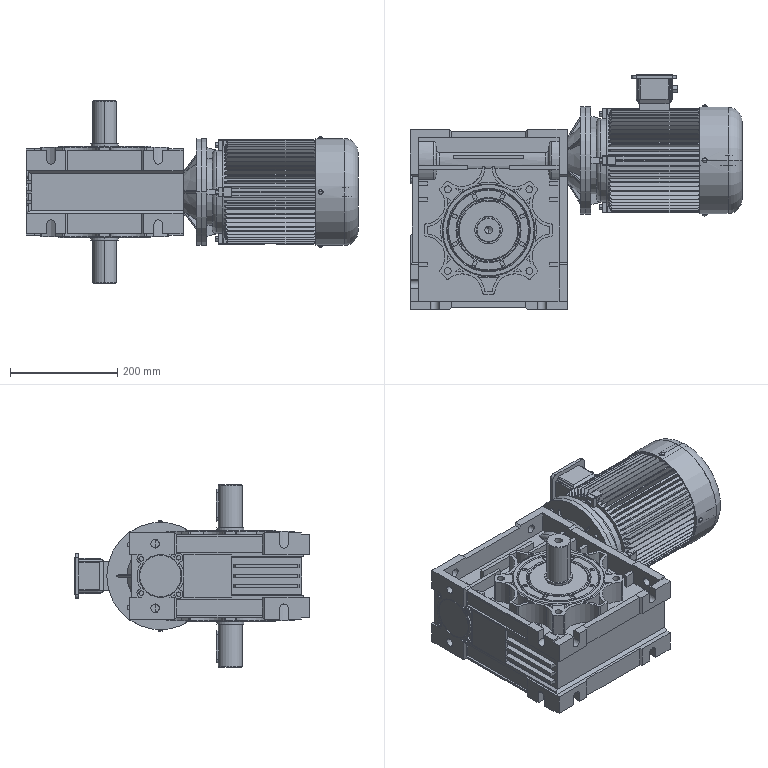Part | SolidWorks | 4 solids | 1490 faces | box 618.25 x 437.5 x 340 mm | volume 18932676 mm3 | plane 882 | cylinder 368 | cone 190 | torus 42 | sphere 8 | commonest cylinder face diameters 5.184 x42 85.927 x36 16 x28 178.45 x26 75.559 x20 12.8 x16